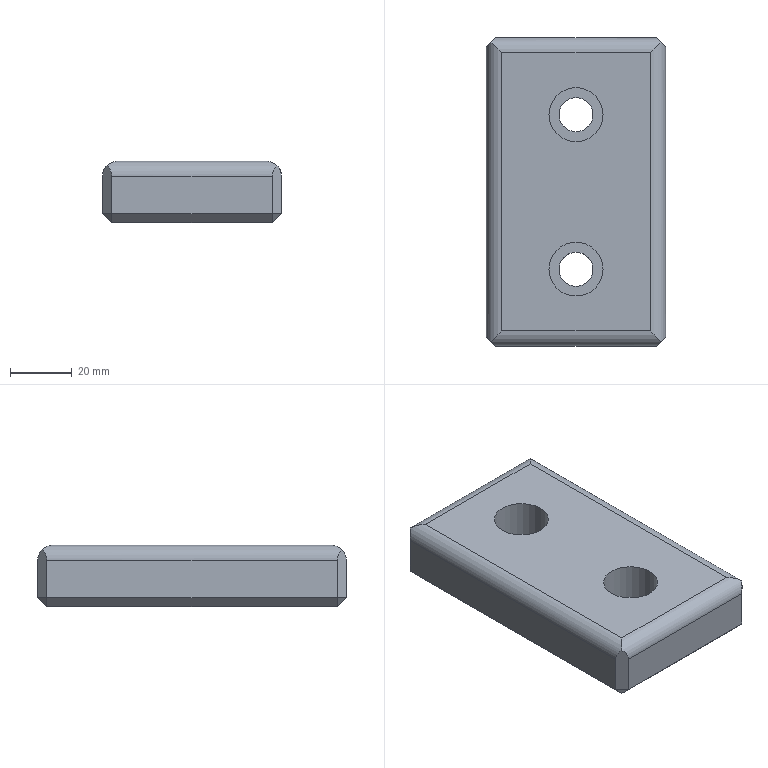Part | NX | features MAIN_BODY 2 | 1 solid | 28 faces | box 58 x 100 x 20 mm | volume 105403 mm3 | plane 20 | cylinder 8 | commonest cylinder face diameters 10 x4 11 x2 17.5 x2
STEP:
#1=CARTESIAN_POINT('',(-590.,-80.,-377.));
#2=VERTEX_POINT('',#1);
#3=CARTESIAN_POINT('',(-590.,-80.,-365.));
#4=VERTEX_POINT('',#3);
#5=CARTESIAN_POINT('',(-590.,-80.,-360.));
#6=DIRECTION('',(0.,0.,1.));
#7=VECTOR('',#6,1000.);
#8=LINE('',#5,#7);
#9=EDGE_CURVE('',#2,#4,#8,.T.);
#10=ORIENTED_EDGE('',*,*,#9,.T.);
#11=CARTESIAN_POINT('',(-538.,-80.,-365.));
#12=VERTEX_POINT('',#11);
#13=CARTESIAN_POINT('',(-538.,-80.,-365.));
#14=DIRECTION('',(1.,0.,0.));
#15=VECTOR('',#14,1000.);
#16=LINE('',#13,#15);
#17=EDGE_CURVE('',#4,#12,#16,.T.);
#18=ORIENTED_EDGE('',*,*,#17,.T.);
#19=CARTESIAN_POINT('',(-538.,-80.,-377.));
#20=VERTEX_POINT('',#19);
#21=CARTESIAN_POINT('',(-538.,-80.,-360.));
#22=DIRECTION('',(0.,0.,-1.));
#23=VECTOR('',#22,1000.);
#24=LINE('',#21,#23);
#25=EDGE_CURVE('',#12,#20,#24,.T.);
#26=ORIENTED_EDGE('',*,*,#25,.T.);
#27=CARTESIAN_POINT('',(-593.,-80.,-377.));
#28=DIRECTION('',(-1.,0.,0.));
#29=VECTOR('',#28,1000.);
#30=LINE('',#27,#29);
#31=EDGE_CURVE('',#20,#2,#30,.T.);
#32=ORIENTED_EDGE('',*,*,#31,.T.);
#33=EDGE_LOOP('',(#10,#18,#26,#32));
#34=FACE_BOUND('',#33,.T.);
#35=CARTESIAN_POINT('',(-593.,-80.,-360.));
#36=DIRECTION('',(0.,1.,0.));
#37=DIRECTION('',(-1.,0.,0.));
#38=AXIS2_PLACEMENT_3D('',#35,#36,#37);
#39=PLANE('',#38);
#40=ADVANCED_FACE('',(#34),#39,.T.);
#41=CARTESIAN_POINT('',(-535.,-83.,-377.));
#42=VERTEX_POINT('',#41);
#43=CARTESIAN_POINT('',(-535.,-83.,-365.));
#44=VERTEX_POINT('',#43);
#45=CARTESIAN_POINT('',(-535.,-83.,-360.));
#46=DIRECTION('',(0.,0.,1.));
#47=VECTOR('',#46,1000.);
#48=LINE('',#45,#47);
#49=EDGE_CURVE('',#42,#44,#48,.T.);
#50=ORIENTED_EDGE('',*,*,#49,.T.);
#51=CARTESIAN_POINT('',(-535.,-177.,-365.));
#52=VERTEX_POINT('',#51);
#53=CARTESIAN_POINT('',(-535.,-177.,-365.));
#54=DIRECTION('',(0.,-1.,0.));
#55=VECTOR('',#54,1000.);
#56=LINE('',#53,#55);
#57=EDGE_CURVE('',#44,#52,#56,.T.);
#58=ORIENTED_EDGE('',*,*,#57,.T.);
#59=CARTESIAN_POINT('',(-535.,-177.,-377.));
#60=VERTEX_POINT('',#59);
#61=CARTESIAN_POINT('',(-535.,-177.,-360.));
#62=DIRECTION('',(0.,0.,-1.));
#63=VECTOR('',#62,1000.);
#64=LINE('',#61,#63);
#65=EDGE_CURVE('',#52,#60,#64,.T.);
#66=ORIENTED_EDGE('',*,*,#65,.T.);
#67=CARTESIAN_POINT('',(-535.,-80.,-377.));
#68=DIRECTION('',(0.,1.,0.));
#69=VECTOR('',#68,1000.);
#70=LINE('',#67,#69);
#71=EDGE_CURVE('',#60,#42,#70,.T.);
#72=ORIENTED_EDGE('',*,*,#71,.T.);
#73=EDGE_LOOP('',(#50,#58,#66,#72));
#74=FACE_BOUND('',#73,.T.);
#75=CARTESIAN_POINT('',(-535.,-80.,-360.));
#76=DIRECTION('',(1.,0.,0.));
#77=DIRECTION('',(0.,1.,0.));
#78=AXIS2_PLACEMENT_3D('',#75,#76,#77);
#79=PLANE('',#78);
#80=ADVANCED_FACE('',(#74),#79,.T.);
#81=CARTESIAN_POINT('',(-538.,-180.,-377.));
#82=VERTEX_POINT('',#81);
#83=CARTESIAN_POINT('',(-538.,-180.,-365.));
#84=VERTEX_POINT('',#83);
#85=CARTESIAN_POINT('',(-538.,-180.,-360.));
#86=DIRECTION('',(0.,0.,1.));
#87=VECTOR('',#86,1000.);
#88=LINE('',#85,#87);
#89=EDGE_CURVE('',#82,#84,#88,.T.);
#90=ORIENTED_EDGE('',*,*,#89,.T.);
#91=CARTESIAN_POINT('',(-590.,-180.,-365.));
#92=VERTEX_POINT('',#91);
#93=CARTESIAN_POINT('',(-590.,-180.,-365.));
#94=DIRECTION('',(-1.,0.,0.));
#95=VECTOR('',#94,1000.);
#96=LINE('',#93,#95);
#97=EDGE_CURVE('',#84,#92,#96,.T.);
#98=ORIENTED_EDGE('',*,*,#97,.T.);
#99=CARTESIAN_POINT('',(-590.,-180.,-377.));
#100=VERTEX_POINT('',#99);
#101=CARTESIAN_POINT('',(-590.,-180.,-360.));
#102=DIRECTION('',(0.,0.,-1.));
#103=VECTOR('',#102,1000.);
#104=LINE('',#101,#103);
#105=EDGE_CURVE('',#92,#100,#104,.T.);
#106=ORIENTED_EDGE('',*,*,#105,.T.);
#107=CARTESIAN_POINT('',(-535.,-180.,-377.));
#108=DIRECTION('',(1.,0.,0.));
#109=VECTOR('',#108,1000.);
#110=LINE('',#107,#109);
#111=EDGE_CURVE('',#100,#82,#110,.T.);
#112=ORIENTED_EDGE('',*,*,#111,.T.);
#113=EDGE_LOOP('',(#90,#98,#106,#112));
#114=FACE_BOUND('',#113,.T.);
#115=CARTESIAN_POINT('',(-535.,-180.,-360.));
#116=DIRECTION('',(0.,-1.,0.));
#117=DIRECTION('',(0.,0.,1.));
#118=AXIS2_PLACEMENT_3D('',#115,#116,#117);
#119=PLANE('',#118);
#120=ADVANCED_FACE('',(#114),#119,.T.);
#121=CARTESIAN_POINT('',(-593.,-177.,-377.));
#122=VERTEX_POINT('',#121);
#123=CARTESIAN_POINT('',(-593.,-177.,-365.));
#124=VERTEX_POINT('',#123);
#125=CARTESIAN_POINT('',(-593.,-177.,-360.));
#126=DIRECTION('',(0.,0.,1.));
#127=VECTOR('',#126,1000.);
#128=LINE('',#125,#127);
#129=EDGE_CURVE('',#122,#124,#128,.T.);
#130=ORIENTED_EDGE('',*,*,#129,.T.);
#131=CARTESIAN_POINT('',(-593.,-83.,-365.));
#132=VERTEX_POINT('',#131);
#133=CARTESIAN_POINT('',(-593.,-83.,-365.));
#134=DIRECTION('',(0.,1.,0.));
#135=VECTOR('',#134,1000.);
#136=LINE('',#133,#135);
#137=EDGE_CURVE('',#124,#132,#136,.T.);
#138=ORIENTED_EDGE('',*,*,#137,.T.);
#139=CARTESIAN_POINT('',(-593.,-83.,-377.));
#140=VERTEX_POINT('',#139);
#141=CARTESIAN_POINT('',(-593.,-83.,-360.));
#142=DIRECTION('',(0.,0.,-1.));
#143=VECTOR('',#142,1000.);
#144=LINE('',#141,#143);
#145=EDGE_CURVE('',#132,#140,#144,.T.);
#146=ORIENTED_EDGE('',*,*,#145,.T.);
#147=CARTESIAN_POINT('',(-593.,-180.,-377.));
#148=DIRECTION('',(0.,-1.,0.));
#149=VECTOR('',#148,1000.);
#150=LINE('',#147,#149);
#151=EDGE_CURVE('',#140,#122,#150,.T.);
#152=ORIENTED_EDGE('',*,*,#151,.T.);
#153=EDGE_LOOP('',(#130,#138,#146,#152));
#154=FACE_BOUND('',#153,.T.);
#155=CARTESIAN_POINT('',(-593.,-180.,-360.));
#156=DIRECTION('',(-1.,0.,0.));
#157=DIRECTION('',(0.,-1.,0.));
#158=AXIS2_PLACEMENT_3D('',#155,#156,#157);
#159=PLANE('',#158);
#160=ADVANCED_FACE('',(#154),#159,.T.);
#161=CARTESIAN_POINT('',(-540.,-175.,-360.));
#162=VERTEX_POINT('',#161);
#163=CARTESIAN_POINT('',(-540.,-85.,-360.));
#164=VERTEX_POINT('',#163);
#165=CARTESIAN_POINT('',(-540.,-83.,-360.));
#166=DIRECTION('',(0.,-1.,0.));
#167=VECTOR('',#166,1000.);
#168=LINE('',#165,#167);
#169=EDGE_CURVE('',#162,#164,#168,.F.);
#170=ORIENTED_EDGE('',*,*,#169,.T.);
#171=CARTESIAN_POINT('',(-588.,-85.,-360.));
#172=VERTEX_POINT('',#171);
#173=CARTESIAN_POINT('',(-590.,-85.,-360.));
#174=DIRECTION('',(1.,0.,0.));
#175=VECTOR('',#174,1000.);
#176=LINE('',#173,#175);
#177=EDGE_CURVE('',#164,#172,#176,.F.);
#178=ORIENTED_EDGE('',*,*,#177,.T.);
#179=CARTESIAN_POINT('',(-588.,-175.,-360.));
#180=VERTEX_POINT('',#179);
#181=CARTESIAN_POINT('',(-588.,-177.,-360.));
#182=DIRECTION('',(0.,1.,0.));
#183=VECTOR('',#182,1000.);
#184=LINE('',#181,#183);
#185=EDGE_CURVE('',#172,#180,#184,.F.);
#186=ORIENTED_EDGE('',*,*,#185,.T.);
#187=CARTESIAN_POINT('',(-538.,-175.,-360.));
#188=DIRECTION('',(-1.,0.,0.));
#189=VECTOR('',#188,1000.);
#190=LINE('',#187,#189);
#191=EDGE_CURVE('',#180,#162,#190,.F.);
#192=ORIENTED_EDGE('',*,*,#191,.T.);
#193=EDGE_LOOP('',(#170,#178,#186,#192));
#194=FACE_BOUND('',#193,.T.);
#195=CARTESIAN_POINT('',(-555.25,-155.,-360.));
#196=VERTEX_POINT('',#195);
#197=CARTESIAN_POINT('',(-564.,-155.,-360.));
#198=DIRECTION('',(0.,0.,-1.));
#199=DIRECTION('',(1.,0.,0.));
#200=AXIS2_PLACEMENT_3D('',#197,#198,#199);
#201=CIRCLE('',#200,8.75);
#202=EDGE_CURVE('',#196,#196,#201,.T.);
#203=ORIENTED_EDGE('',*,*,#202,.T.);
#204=EDGE_LOOP('',(#203));
#205=FACE_BOUND('',#204,.T.);
#206=CARTESIAN_POINT('',(-555.25,-105.,-360.));
#207=VERTEX_POINT('',#206);
#208=CARTESIAN_POINT('',(-564.,-105.,-360.));
#209=DIRECTION('',(0.,0.,-1.));
#210=DIRECTION('',(1.,0.,0.));
#211=AXIS2_PLACEMENT_3D('',#208,#209,#210);
#212=CIRCLE('',#211,8.75);
#213=EDGE_CURVE('',#207,#207,#212,.T.);
#214=ORIENTED_EDGE('',*,*,#213,.T.);
#215=EDGE_LOOP('',(#214));
#216=FACE_BOUND('',#215,.T.);
#217=CARTESIAN_POINT('',(-535.,-80.,-360.));
#218=DIRECTION('',(0.,0.,-1.));
#219=DIRECTION('',(1.,0.,0.));
#220=AXIS2_PLACEMENT_3D('',#217,#218,#219);
#221=PLANE('',#220);
#222=ADVANCED_FACE('',(#194,#205,#216),#221,.F.);
#223=CARTESIAN_POINT('',(-590.,-83.,-380.));
#224=VERTEX_POINT('',#223);
#225=CARTESIAN_POINT('',(-538.,-83.,-380.));
#226=VERTEX_POINT('',#225);
#227=CARTESIAN_POINT('',(-535.,-83.,-380.));
#228=DIRECTION('',(1.,0.,0.));
#229=VECTOR('',#228,1000.);
#230=LINE('',#227,#229);
#231=EDGE_CURVE('',#224,#226,#230,.T.);
#232=ORIENTED_EDGE('',*,*,#231,.T.);
#233=CARTESIAN_POINT('',(-538.,-177.,-380.));
#234=VERTEX_POINT('',#233);
#235=CARTESIAN_POINT('',(-538.,-80.,-380.));
#236=DIRECTION('',(0.,-1.,0.));
#237=VECTOR('',#236,1000.);
#238=LINE('',#235,#237);
#239=EDGE_CURVE('',#226,#234,#238,.T.);
#240=ORIENTED_EDGE('',*,*,#239,.T.);
#241=CARTESIAN_POINT('',(-590.,-177.,-380.));
#242=VERTEX_POINT('',#241);
#243=CARTESIAN_POINT('',(-535.,-177.,-380.));
#244=DIRECTION('',(-1.,0.,0.));
#245=VECTOR('',#244,1000.);
#246=LINE('',#243,#245);
#247=EDGE_CURVE('',#234,#242,#246,.T.);
#248=ORIENTED_EDGE('',*,*,#247,.T.);
#249=CARTESIAN_POINT('',(-590.,-80.,-380.));
#250=DIRECTION('',(0.,1.,0.));
#251=VECTOR('',#250,1000.);
#252=LINE('',#249,#251);
#253=EDGE_CURVE('',#242,#224,#252,.T.);
#254=ORIENTED_EDGE('',*,*,#253,.T.);
#255=EDGE_LOOP('',(#232,#240,#248,#254));
#256=FACE_BOUND('',#255,.T.);
#257=CARTESIAN_POINT('',(-558.5,-155.,-380.));
#258=VERTEX_POINT('',#257);
#259=CARTESIAN_POINT('',(-564.,-155.,-380.));
#260=DIRECTION('',(0.,0.,-1.));
#261=DIRECTION('',(1.,0.,0.));
#262=AXIS2_PLACEMENT_3D('',#259,#260,#261);
#263=CIRCLE('',#262,5.5);
#264=EDGE_CURVE('',#258,#258,#263,.T.);
#265=ORIENTED_EDGE('',*,*,#264,.F.);
#266=EDGE_LOOP('',(#265));
#267=FACE_BOUND('',#266,.T.);
#268=CARTESIAN_POINT('',(-558.5,-105.,-380.));
#269=VERTEX_POINT('',#268);
#270=CARTESIAN_POINT('',(-564.,-105.,-380.));
#271=DIRECTION('',(0.,0.,-1.));
#272=DIRECTION('',(1.,0.,0.));
#273=AXIS2_PLACEMENT_3D('',#270,#271,#272);
#274=CIRCLE('',#273,5.5);
#275=EDGE_CURVE('',#269,#269,#274,.T.);
#276=ORIENTED_EDGE('',*,*,#275,.F.);
#277=EDGE_LOOP('',(#276));
#278=FACE_BOUND('',#277,.T.);
#279=CARTESIAN_POINT('',(-535.,-80.,-380.));
#280=DIRECTION('',(0.,0.,-1.));
#281=DIRECTION('',(1.,0.,0.));
#282=AXIS2_PLACEMENT_3D('',#279,#280,#281);
#283=PLANE('',#282);
#284=ADVANCED_FACE('',(#256,#267,#278),#283,.T.);
#285=ORIENTED_EDGE('',*,*,#275,.T.);
#286=EDGE_LOOP('',(#285));
#287=FACE_BOUND('',#286,.T.);
#288=CARTESIAN_POINT('',(-558.5,-105.,-372.));
#289=VERTEX_POINT('',#288);
#290=CARTESIAN_POINT('',(-564.,-105.,-372.));
#291=DIRECTION('',(0.,0.,-1.));
#292=DIRECTION('',(1.,0.,0.));
#293=AXIS2_PLACEMENT_3D('',#290,#291,#292);
#294=CIRCLE('',#293,5.5);
#295=EDGE_CURVE('',#289,#289,#294,.T.);
#296=ORIENTED_EDGE('',*,*,#295,.F.);
#297=EDGE_LOOP('',(#296));
#298=FACE_BOUND('',#297,.T.);
#299=CARTESIAN_POINT('',(-564.,-105.,-410.));
#300=DIRECTION('',(0.,0.,-1.));
#301=DIRECTION('',(1.,0.,0.));
#302=AXIS2_PLACEMENT_3D('',#299,#300,#301);
#303=CYLINDRICAL_SURFACE('',#302,5.5);
#304=ADVANCED_FACE('',(#287,#298),#303,.F.);
#305=ORIENTED_EDGE('',*,*,#295,.T.);
#306=EDGE_LOOP('',(#305));
#307=FACE_BOUND('',#306,.T.);
#308=CARTESIAN_POINT('',(-555.25,-105.,-372.));
#309=VERTEX_POINT('',#308);
#310=CARTESIAN_POINT('',(-564.,-105.,-372.));
#311=DIRECTION('',(0.,0.,-1.));
#312=DIRECTION('',(1.,0.,0.));
#313=AXIS2_PLACEMENT_3D('',#310,#311,#312);
#314=CIRCLE('',#313,8.75);
#315=EDGE_CURVE('',#309,#309,#314,.T.);
#316=ORIENTED_EDGE('',*,*,#315,.F.);
#317=EDGE_LOOP('',(#316));
#318=FACE_BOUND('',#317,.T.);
#319=CARTESIAN_POINT('',(-564.,-105.,-372.));
#320=DIRECTION('',(0.,0.,-1.));
#321=DIRECTION('',(1.,0.,0.));
#322=AXIS2_PLACEMENT_3D('',#319,#320,#321);
#323=PLANE('',#322);
#324=ADVANCED_FACE('',(#307,#318),#323,.F.);
#325=ORIENTED_EDGE('',*,*,#315,.T.);
#326=EDGE_LOOP('',(#325));
#327=FACE_BOUND('',#326,.T.);
#328=ORIENTED_EDGE('',*,*,#213,.F.);
#329=EDGE_LOOP('',(#328));
#330=FACE_BOUND('',#329,.T.);
#331=CARTESIAN_POINT('',(-564.,-105.,-360.));
#332=DIRECTION('',(0.,0.,-1.));
#333=DIRECTION('',(1.,0.,0.));
#334=AXIS2_PLACEMENT_3D('',#331,#332,#333);
#335=CYLINDRICAL_SURFACE('',#334,8.75);
#336=ADVANCED_FACE('',(#327,#330),#335,.F.);
#337=ORIENTED_EDGE('',*,*,#264,.T.);
#338=EDGE_LOOP('',(#337));
#339=FACE_BOUND('',#338,.T.);
#340=CARTESIAN_POINT('',(-558.5,-155.,-372.));
#341=VERTEX_POINT('',#340);
#342=CARTESIAN_POINT('',(-564.,-155.,-372.));
#343=DIRECTION('',(0.,0.,-1.));
#344=DIRECTION('',(1.,0.,0.));
#345=AXIS2_PLACEMENT_3D('',#342,#343,#344);
#346=CIRCLE('',#345,5.5);
#347=EDGE_CURVE('',#341,#341,#346,.T.);
#348=ORIENTED_EDGE('',*,*,#347,.F.);
#349=EDGE_LOOP('',(#348));
#350=FACE_BOUND('',#349,.T.);
#351=CARTESIAN_POINT('',(-564.,-155.,-410.));
#352=DIRECTION('',(0.,0.,-1.));
#353=DIRECTION('',(1.,0.,0.));
#354=AXIS2_PLACEMENT_3D('',#351,#352,#353);
#355=CYLINDRICAL_SURFACE('',#354,5.5);
#356=ADVANCED_FACE('',(#339,#350),#355,.F.);
#357=ORIENTED_EDGE('',*,*,#347,.T.);
#358=EDGE_LOOP('',(#357));
#359=FACE_BOUND('',#358,.T.);
#360=CARTESIAN_POINT('',(-555.25,-155.,-372.));
#361=VERTEX_POINT('',#360);
#362=CARTESIAN_POINT('',(-564.,-155.,-372.));
#363=DIRECTION('',(0.,0.,-1.));
#364=DIRECTION('',(1.,0.,0.));
#365=AXIS2_PLACEMENT_3D('',#362,#363,#364);
#366=CIRCLE('',#365,8.75);
#367=EDGE_CURVE('',#361,#361,#366,.T.);
#368=ORIENTED_EDGE('',*,*,#367,.F.);
#369=EDGE_LOOP('',(#368));
#370=FACE_BOUND('',#369,.T.);
#371=CARTESIAN_POINT('',(-564.,-155.,-372.));
#372=DIRECTION('',(0.,0.,-1.));
#373=DIRECTION('',(1.,0.,0.));
#374=AXIS2_PLACEMENT_3D('',#371,#372,#373);
#375=PLANE('',#374);
#376=ADVANCED_FACE('',(#359,#370),#375,.F.);
#377=ORIENTED_EDGE('',*,*,#367,.T.);
#378=EDGE_LOOP('',(#377));
#379=FACE_BOUND('',#378,.T.);
#380=ORIENTED_EDGE('',*,*,#202,.F.);
#381=EDGE_LOOP('',(#380));
#382=FACE_BOUND('',#381,.T.);
#383=CARTESIAN_POINT('',(-564.,-155.,-360.));
#384=DIRECTION('',(0.,0.,-1.));
#385=DIRECTION('',(1.,0.,0.));
#386=AXIS2_PLACEMENT_3D('',#383,#384,#385);
#387=CYLINDRICAL_SURFACE('',#386,8.75);
#388=ADVANCED_FACE('',(#379,#382),#387,.F.);
#389=CARTESIAN_POINT('',(-591.5,-81.5,-361.429));
#390=VERTEX_POINT('',#389);
#391=CARTESIAN_POINT('',(-588.,-78.,-365.));
#392=DIRECTION('',(0.7071,-0.7071,0.));
#393=DIRECTION('',(-0.7071,-0.7071,0.));
#394=AXIS2_PLACEMENT_3D('',#391,#392,#393);
#395=ELLIPSE('',#394,7.071,5.);
#396=EDGE_CURVE('',#132,#390,#395,.F.);
#397=ORIENTED_EDGE('',*,*,#396,.T.);
#398=CARTESIAN_POINT('',(-595.,-85.,-365.));
#399=DIRECTION('',(0.7071,-0.7071,0.));
#400=DIRECTION('',(-0.7071,-0.7071,0.));
#401=AXIS2_PLACEMENT_3D('',#398,#399,#400);
#402=ELLIPSE('',#401,7.071,5.);
#403=EDGE_CURVE('',#390,#4,#402,.F.);
#404=ORIENTED_EDGE('',*,*,#403,.T.);
#405=ORIENTED_EDGE('',*,*,#9,.F.);
#406=CARTESIAN_POINT('',(-591.5,-81.5,-377.));
#407=DIRECTION('',(-0.7071,-0.7071,0.));
#408=VECTOR('',#407,1000.);
#409=LINE('',#406,#408);
#410=EDGE_CURVE('',#140,#2,#409,.F.);
#411=ORIENTED_EDGE('',*,*,#410,.F.);
#412=ORIENTED_EDGE('',*,*,#145,.F.);
#413=EDGE_LOOP('',(#397,#404,#405,#411,#412));
#414=FACE_BOUND('',#413,.T.);
#415=CARTESIAN_POINT('',(-593.,-83.,-360.));
#416=DIRECTION('',(0.7071,-0.7071,0.));
#417=DIRECTION('',(0.7071,0.7071,0.));
#418=AXIS2_PLACEMENT_3D('',#415,#416,#417);
#419=PLANE('',#418);
#420=ADVANCED_FACE('',(#414),#419,.F.);
#421=CARTESIAN_POINT('',(-590.,-177.,-380.));
#422=DIRECTION('',(-0.7071,0.,0.7071));
#423=VECTOR('',#422,1000.);
#424=LINE('',#421,#423);
#425=EDGE_CURVE('',#122,#242,#424,.F.);
#426=ORIENTED_EDGE('',*,*,#425,.F.);
#427=ORIENTED_EDGE('',*,*,#151,.F.);
#428=CARTESIAN_POINT('',(-590.,-83.,-380.));
#429=DIRECTION('',(0.7071,0.,-0.7071));
#430=VECTOR('',#429,1000.);
#431=LINE('',#428,#430);
#432=EDGE_CURVE('',#224,#140,#431,.F.);
#433=ORIENTED_EDGE('',*,*,#432,.F.);
#434=ORIENTED_EDGE('',*,*,#253,.F.);
#435=EDGE_LOOP('',(#426,#427,#433,#434));
#436=FACE_BOUND('',#435,.T.);
#437=CARTESIAN_POINT('',(-590.,-80.,-380.));
#438=DIRECTION('',(0.7071,0.,0.7071));
#439=DIRECTION('',(-0.7071,0.,0.7071));
#440=AXIS2_PLACEMENT_3D('',#437,#438,#439);
#441=PLANE('',#440);
#442=ADVANCED_FACE('',(#436),#441,.F.);
#443=ORIENTED_EDGE('',*,*,#105,.F.);
#444=CARTESIAN_POINT('',(-591.5,-178.5,-361.429));
#445=VERTEX_POINT('',#444);
#446=CARTESIAN_POINT('',(-595.,-175.,-365.));
#447=DIRECTION('',(0.7071,0.7071,0.));
#448=DIRECTION('',(0.7071,-0.7071,0.));
#449=AXIS2_PLACEMENT_3D('',#446,#447,#448);
#450=ELLIPSE('',#449,7.071,5.);
#451=EDGE_CURVE('',#92,#445,#450,.F.);
#452=ORIENTED_EDGE('',*,*,#451,.T.);
#453=CARTESIAN_POINT('',(-588.,-182.,-365.));
#454=DIRECTION('',(0.7071,0.7071,0.));
#455=DIRECTION('',(0.7071,-0.7071,0.));
#456=AXIS2_PLACEMENT_3D('',#453,#454,#455);
#457=ELLIPSE('',#456,7.071,5.);
#458=EDGE_CURVE('',#445,#124,#457,.F.);
#459=ORIENTED_EDGE('',*,*,#458,.T.);
#460=ORIENTED_EDGE('',*,*,#129,.F.);
#461=CARTESIAN_POINT('',(-591.5,-178.5,-377.));
#462=DIRECTION('',(0.7071,-0.7071,0.));
#463=VECTOR('',#462,1000.);
#464=LINE('',#461,#463);
#465=EDGE_CURVE('',#100,#122,#464,.F.);
#466=ORIENTED_EDGE('',*,*,#465,.F.);
#467=EDGE_LOOP('',(#443,#452,#459,#460,#466));
#468=FACE_BOUND('',#467,.T.);
#469=CARTESIAN_POINT('',(-590.,-180.,-360.));
#470=DIRECTION('',(0.7071,0.7071,0.));
#471=DIRECTION('',(-0.7071,0.7071,0.));
#472=AXIS2_PLACEMENT_3D('',#469,#470,#471);
#473=PLANE('',#472);
#474=ADVANCED_FACE('',(#468),#473,.F.);
#475=ORIENTED_EDGE('',*,*,#432,.T.);
#476=ORIENTED_EDGE('',*,*,#410,.T.);
#477=CARTESIAN_POINT('',(-590.,-83.,-380.));
#478=DIRECTION('',(0.,0.7071,0.7071));
#479=VECTOR('',#478,1000.);
#480=LINE('',#477,#479);
#481=EDGE_CURVE('',#224,#2,#480,.T.);
#482=ORIENTED_EDGE('',*,*,#481,.F.);
#483=EDGE_LOOP('',(#475,#476,#482));
#484=FACE_BOUND('',#483,.T.);
#485=CARTESIAN_POINT('',(-590.,-83.,-380.));
#486=DIRECTION('',(-0.5774,0.5774,-0.5774));
#487=DIRECTION('',(0.,-0.7071,-0.7071));
#488=AXIS2_PLACEMENT_3D('',#485,#486,#487);
#489=PLANE('',#488);
#490=ADVANCED_FACE('',(#484),#489,.T.);
#491=ORIENTED_EDGE('',*,*,#465,.T.);
#492=ORIENTED_EDGE('',*,*,#425,.T.);
#493=CARTESIAN_POINT('',(-590.,-177.,-380.));
#494=DIRECTION('',(0.,0.7071,-0.7071));
#495=VECTOR('',#494,1000.);
#496=LINE('',#493,#495);
#497=EDGE_CURVE('',#100,#242,#496,.T.);
#498=ORIENTED_EDGE('',*,*,#497,.F.);
#499=EDGE_LOOP('',(#491,#492,#498));
#500=FACE_BOUND('',#499,.T.);
#501=CARTESIAN_POINT('',(-590.,-177.,-380.));
#502=DIRECTION('',(-0.5774,-0.5774,-0.5774));
#503=DIRECTION('',(0.7071,0.,-0.7071));
#504=AXIS2_PLACEMENT_3D('',#501,#502,#503);
#505=PLANE('',#504);
#506=ADVANCED_FACE('',(#500),#505,.T.);
#507=ORIENTED_EDGE('',*,*,#25,.F.);
#508=CARTESIAN_POINT('',(-536.5,-81.5,-361.429));
#509=VERTEX_POINT('',#508);
#510=CARTESIAN_POINT('',(-533.,-85.,-365.));
#511=DIRECTION('',(-0.7071,-0.7071,0.));
#512=DIRECTION('',(-0.7071,0.7071,0.));
#513=AXIS2_PLACEMENT_3D('',#510,#511,#512);
#514=ELLIPSE('',#513,7.071,5.);
#515=EDGE_CURVE('',#12,#509,#514,.F.);
#516=ORIENTED_EDGE('',*,*,#515,.T.);
#517=CARTESIAN_POINT('',(-540.,-78.,-365.));
#518=DIRECTION('',(-0.7071,-0.7071,0.));
#519=DIRECTION('',(-0.7071,0.7071,0.));
#520=AXIS2_PLACEMENT_3D('',#517,#518,#519);
#521=ELLIPSE('',#520,7.071,5.);
#522=EDGE_CURVE('',#509,#44,#521,.F.);
#523=ORIENTED_EDGE('',*,*,#522,.T.);
#524=ORIENTED_EDGE('',*,*,#49,.F.);
#525=CARTESIAN_POINT('',(-535.,-83.,-377.));
#526=DIRECTION('',(-0.7071,0.7071,0.));
#527=VECTOR('',#526,1000.);
#528=LINE('',#525,#527);
#529=EDGE_CURVE('',#20,#42,#528,.F.);
#530=ORIENTED_EDGE('',*,*,#529,.F.);
#531=EDGE_LOOP('',(#507,#516,#523,#524,#530));
#532=FACE_BOUND('',#531,.T.);
#533=CARTESIAN_POINT('',(-538.,-80.,-360.));
#534=DIRECTION('',(-0.7071,-0.7071,0.));
#535=DIRECTION('',(0.7071,-0.7071,0.));
#536=AXIS2_PLACEMENT_3D('',#533,#534,#535);
#537=PLANE('',#536);
#538=ADVANCED_FACE('',(#532),#537,.F.);
#539=ORIENTED_EDGE('',*,*,#481,.T.);
#540=ORIENTED_EDGE('',*,*,#31,.F.);
#541=CARTESIAN_POINT('',(-538.,-81.5,-378.5));
#542=DIRECTION('',(0.,-0.7071,-0.7071));
#543=VECTOR('',#542,1000.);
#544=LINE('',#541,#543);
#545=EDGE_CURVE('',#226,#20,#544,.F.);
#546=ORIENTED_EDGE('',*,*,#545,.F.);
#547=ORIENTED_EDGE('',*,*,#231,.F.);
#548=EDGE_LOOP('',(#539,#540,#546,#547));
#549=FACE_BOUND('',#548,.T.);
#550=CARTESIAN_POINT('',(-535.,-83.,-380.));
#551=DIRECTION('',(0.,-0.7071,0.7071));
#552=DIRECTION('',(0.,0.7071,0.7071));
#553=AXIS2_PLACEMENT_3D('',#550,#551,#552);
#554=PLANE('',#553);
#555=ADVANCED_FACE('',(#549),#554,.F.);
#556=ORIENTED_EDGE('',*,*,#497,.T.);
#557=ORIENTED_EDGE('',*,*,#247,.F.);
#558=CARTESIAN_POINT('',(-538.,-177.,-380.));
#559=DIRECTION('',(0.,-0.7071,0.7071));
#560=VECTOR('',#559,1000.);
#561=LINE('',#558,#560);
#562=EDGE_CURVE('',#82,#234,#561,.F.);
#563=ORIENTED_EDGE('',*,*,#562,.F.);
#564=ORIENTED_EDGE('',*,*,#111,.F.);
#565=EDGE_LOOP('',(#556,#557,#563,#564));
#566=FACE_BOUND('',#565,.T.);
#567=CARTESIAN_POINT('',(-535.,-177.,-380.));
#568=DIRECTION('',(0.,0.7071,0.7071));
#569=DIRECTION('',(0.,0.7071,-0.7071));
#570=AXIS2_PLACEMENT_3D('',#567,#568,#569);
#571=PLANE('',#570);
#572=ADVANCED_FACE('',(#566),#571,.F.);
#573=ORIENTED_EDGE('',*,*,#65,.F.);
#574=CARTESIAN_POINT('',(-536.5,-178.5,-361.429));
#575=VERTEX_POINT('',#574);
#576=CARTESIAN_POINT('',(-540.,-182.,-365.));
#577=DIRECTION('',(-0.7071,0.7071,0.));
#578=DIRECTION('',(0.7071,0.7071,0.));
#579=AXIS2_PLACEMENT_3D('',#576,#577,#578);
#580=ELLIPSE('',#579,7.071,5.);
#581=EDGE_CURVE('',#52,#575,#580,.F.);
#582=ORIENTED_EDGE('',*,*,#581,.T.);
#583=CARTESIAN_POINT('',(-533.,-175.,-365.));
#584=DIRECTION('',(-0.7071,0.7071,0.));
#585=DIRECTION('',(0.7071,0.7071,0.));
#586=AXIS2_PLACEMENT_3D('',#583,#584,#585);
#587=ELLIPSE('',#586,7.071,5.);
#588=EDGE_CURVE('',#575,#84,#587,.F.);
#589=ORIENTED_EDGE('',*,*,#588,.T.);
#590=ORIENTED_EDGE('',*,*,#89,.F.);
#591=CARTESIAN_POINT('',(-536.5,-178.5,-377.));
#592=DIRECTION('',(0.7071,0.7071,0.));
#593=VECTOR('',#592,1000.);
#594=LINE('',#591,#593);
#595=EDGE_CURVE('',#60,#82,#594,.F.);
#596=ORIENTED_EDGE('',*,*,#595,.F.);
#597=EDGE_LOOP('',(#573,#582,#589,#590,#596));
#598=FACE_BOUND('',#597,.T.);
#599=CARTESIAN_POINT('',(-535.,-177.,-360.));
#600=DIRECTION('',(-0.7071,0.7071,0.));
#601=DIRECTION('',(-0.7071,-0.7071,0.));
#602=AXIS2_PLACEMENT_3D('',#599,#600,#601);
#603=PLANE('',#602);
#604=ADVANCED_FACE('',(#598),#603,.F.);
#605=ORIENTED_EDGE('',*,*,#545,.T.);
#606=ORIENTED_EDGE('',*,*,#529,.T.);
#607=CARTESIAN_POINT('',(-535.,-83.,-377.));
#608=DIRECTION('',(0.7071,0.,0.7071));
#609=VECTOR('',#608,1000.);
#610=LINE('',#607,#609);
#611=EDGE_CURVE('',#226,#42,#610,.T.);
#612=ORIENTED_EDGE('',*,*,#611,.F.);
#613=EDGE_LOOP('',(#605,#606,#612));
#614=FACE_BOUND('',#613,.T.);
#615=CARTESIAN_POINT('',(-535.,-83.,-377.));
#616=DIRECTION('',(0.5774,0.5774,-0.5774));
#617=DIRECTION('',(0.7071,0.,0.7071));
#618=AXIS2_PLACEMENT_3D('',#615,#616,#617);
#619=PLANE('',#618);
#620=ADVANCED_FACE('',(#614),#619,.T.);
#621=ORIENTED_EDGE('',*,*,#595,.T.);
#622=ORIENTED_EDGE('',*,*,#562,.T.);
#623=CARTESIAN_POINT('',(-538.,-177.,-380.));
#624=DIRECTION('',(-0.7071,0.,-0.7071));
#625=VECTOR('',#624,1000.);
#626=LINE('',#623,#625);
#627=EDGE_CURVE('',#60,#234,#626,.T.);
#628=ORIENTED_EDGE('',*,*,#627,.F.);
#629=EDGE_LOOP('',(#621,#622,#628));
#630=FACE_BOUND('',#629,.T.);
#631=CARTESIAN_POINT('',(-538.,-177.,-380.));
#632=DIRECTION('',(0.5774,-0.5774,-0.5774));
#633=DIRECTION('',(0.7071,0.,0.7071));
#634=AXIS2_PLACEMENT_3D('',#631,#632,#633);
#635=PLANE('',#634);
#636=ADVANCED_FACE('',(#630),#635,.T.);
#637=ORIENTED_EDGE('',*,*,#611,.T.);
#638=ORIENTED_EDGE('',*,*,#71,.F.);
#639=ORIENTED_EDGE('',*,*,#627,.T.);
#640=ORIENTED_EDGE('',*,*,#239,.F.);
#641=EDGE_LOOP('',(#637,#638,#639,#640));
#642=FACE_BOUND('',#641,.T.);
#643=CARTESIAN_POINT('',(-538.,-80.,-380.));
#644=DIRECTION('',(-0.7071,0.,0.7071));
#645=DIRECTION('',(-0.7071,0.,-0.7071));
#646=AXIS2_PLACEMENT_3D('',#643,#644,#645);
#647=PLANE('',#646);
#648=ADVANCED_FACE('',(#642),#647,.F.);
#649=CARTESIAN_POINT('',(-540.,-175.,-365.));
#650=DIRECTION('',(0.7071,0.7071,0.));
#651=DIRECTION('',(-0.7071,0.7071,0.));
#652=AXIS2_PLACEMENT_3D('',#649,#650,#651);
#653=ELLIPSE('',#652,7.071,5.);
#654=EDGE_CURVE('',#162,#575,#653,.T.);
#655=ORIENTED_EDGE('',*,*,#654,.F.);
#656=ORIENTED_EDGE('',*,*,#191,.F.);
#657=CARTESIAN_POINT('',(-588.,-175.,-365.));
#658=DIRECTION('',(0.7071,-0.7071,0.));
#659=DIRECTION('',(0.7071,0.7071,0.));
#660=AXIS2_PLACEMENT_3D('',#657,#658,#659);
#661=ELLIPSE('',#660,7.071,5.);
#662=EDGE_CURVE('',#445,#180,#661,.F.);
#663=ORIENTED_EDGE('',*,*,#662,.F.);
#664=ORIENTED_EDGE('',*,*,#451,.F.);
#665=ORIENTED_EDGE('',*,*,#97,.F.);
#666=ORIENTED_EDGE('',*,*,#588,.F.);
#667=EDGE_LOOP('',(#655,#656,#663,#664,#665,#666));
#668=FACE_BOUND('',#667,.T.);
#669=CARTESIAN_POINT('',(-535.,-175.,-365.));
#670=DIRECTION('',(1.,0.,0.));
#671=DIRECTION('',(0.,0.,1.));
#672=AXIS2_PLACEMENT_3D('',#669,#670,#671);
#673=CYLINDRICAL_SURFACE('',#672,5.);
#674=ADVANCED_FACE('',(#668),#673,.T.);
#675=ORIENTED_EDGE('',*,*,#662,.T.);
#676=ORIENTED_EDGE('',*,*,#185,.F.);
#677=CARTESIAN_POINT('',(-588.,-85.,-365.));
#678=DIRECTION('',(-0.7071,-0.7071,0.));
#679=DIRECTION('',(0.7071,-0.7071,0.));
#680=AXIS2_PLACEMENT_3D('',#677,#678,#679);
#681=ELLIPSE('',#680,7.071,5.);
#682=EDGE_CURVE('',#390,#172,#681,.F.);
#683=ORIENTED_EDGE('',*,*,#682,.F.);
#684=ORIENTED_EDGE('',*,*,#396,.F.);
#685=ORIENTED_EDGE('',*,*,#137,.F.);
#686=ORIENTED_EDGE('',*,*,#458,.F.);
#687=EDGE_LOOP('',(#675,#676,#683,#684,#685,#686));
#688=FACE_BOUND('',#687,.T.);
#689=CARTESIAN_POINT('',(-588.,-180.,-365.));
#690=DIRECTION('',(0.,-1.,0.));
#691=DIRECTION('',(1.,0.,0.));
#692=AXIS2_PLACEMENT_3D('',#689,#690,#691);
#693=CYLINDRICAL_SURFACE('',#692,5.);
#694=ADVANCED_FACE('',(#688),#693,.T.);
#695=ORIENTED_EDGE('',*,*,#57,.F.);
#696=ORIENTED_EDGE('',*,*,#522,.F.);
#697=CARTESIAN_POINT('',(-540.,-85.,-365.));
#698=DIRECTION('',(-0.7071,0.7071,0.));
#699=DIRECTION('',(-0.7071,-0.7071,0.));
#700=AXIS2_PLACEMENT_3D('',#697,#698,#699);
#701=ELLIPSE('',#700,7.071,5.);
#702=EDGE_CURVE('',#164,#509,#701,.T.);
#703=ORIENTED_EDGE('',*,*,#702,.F.);
#704=ORIENTED_EDGE('',*,*,#169,.F.);
#705=ORIENTED_EDGE('',*,*,#654,.T.);
#706=ORIENTED_EDGE('',*,*,#581,.F.);
#707=EDGE_LOOP('',(#695,#696,#703,#704,#705,#706));
#708=FACE_BOUND('',#707,.T.);
#709=CARTESIAN_POINT('',(-540.,-80.,-365.));
#710=DIRECTION('',(0.,1.,0.));
#711=DIRECTION('',(-1.,0.,0.));
#712=AXIS2_PLACEMENT_3D('',#709,#710,#711);
#713=CYLINDRICAL_SURFACE('',#712,5.);
#714=ADVANCED_FACE('',(#708),#713,.T.);
#715=ORIENTED_EDGE('',*,*,#682,.T.);
#716=ORIENTED_EDGE('',*,*,#177,.F.);
#717=ORIENTED_EDGE('',*,*,#702,.T.);
#718=ORIENTED_EDGE('',*,*,#515,.F.);
#719=ORIENTED_EDGE('',*,*,#17,.F.);
#720=ORIENTED_EDGE('',*,*,#403,.F.);
#721=EDGE_LOOP('',(#715,#716,#717,#718,#719,#720));
#722=FACE_BOUND('',#721,.T.);
#723=CARTESIAN_POINT('',(-593.,-85.,-365.));
#724=DIRECTION('',(-1.,0.,0.));
#725=DIRECTION('',(0.,-1.,0.));
#726=AXIS2_PLACEMENT_3D('',#723,#724,#725);
#727=CYLINDRICAL_SURFACE('',#726,5.);
#728=ADVANCED_FACE('',(#722),#727,.T.);
#729=CLOSED_SHELL('',(#40,#80,#120,#160,#222,#284,#304,#324,#336,#356,#376,#388,#420,#442,#474,#490,#506,#538,#555,#572,#604,#620,#636,#648,#674,#694,#714,#728));
#730=MANIFOLD_SOLID_BREP('',#729);
#731=(LENGTH_UNIT()NAMED_UNIT(*)SI_UNIT(.MILLI.,.METRE.));
#732=UNCERTAINTY_MEASURE_WITH_UNIT(LENGTH_MEASURE(0.00001),#731,'','');
#733=(NAMED_UNIT(*)PLANE_ANGLE_UNIT()SI_UNIT($,.RADIAN.));
#734=(NAMED_UNIT(*)SI_UNIT($,.STERADIAN.)SOLID_ANGLE_UNIT());
#735=(GEOMETRIC_REPRESENTATION_CONTEXT(3)GLOBAL_UNCERTAINTY_ASSIGNED_CONTEXT((#732))GLOBAL_UNIT_ASSIGNED_CONTEXT((#731,#733,#734))REPRESENTATION_CONTEXT('',''));
#736=ADVANCED_BREP_SHAPE_REPRESENTATION('',(#730),#735);